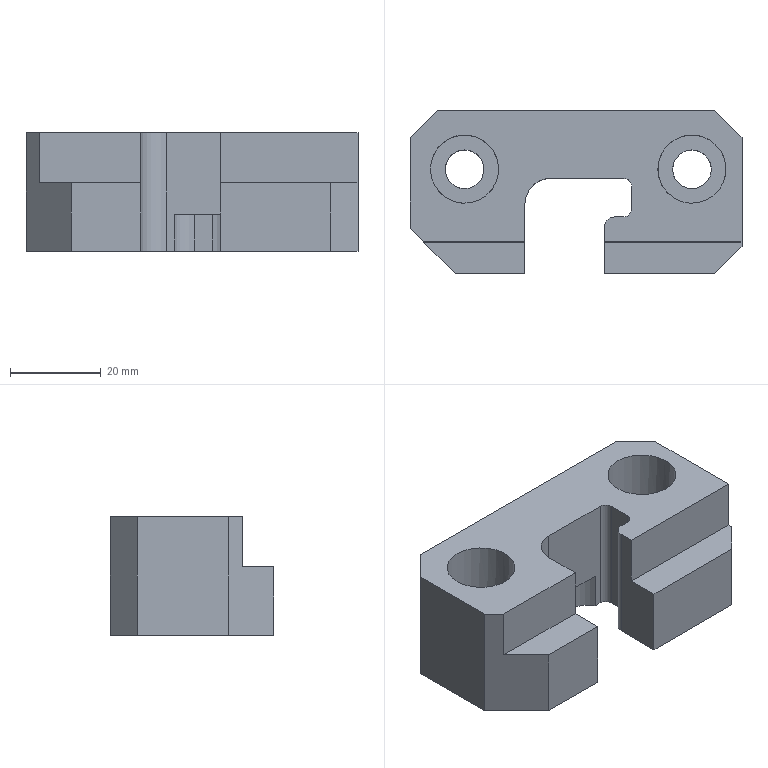Part | STEP file | gslz 2016.10.28-13_id1678_x_t | 1 solid | 34 faces | box 73 x 36 x 26 mm | volume 45297 mm3 | plane 24 | cylinder 10 | commonest cylinder face diameters 3.5 x2 8.5 x2 10 x2 15 x2 4.5 x1 11.5 x1